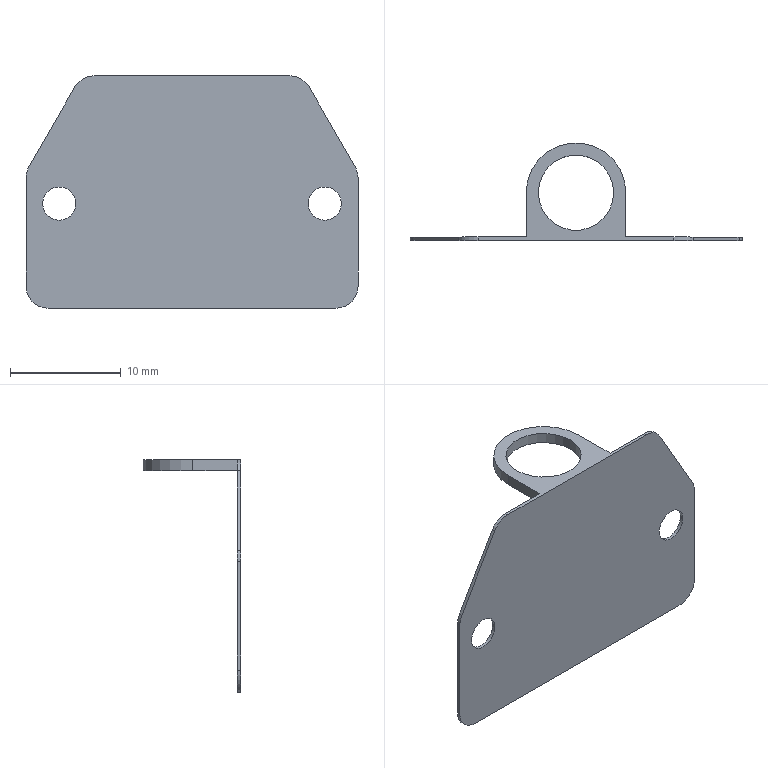Part | STEP file | 1 solid | 21 faces | box 30 x 8.8 x 21 mm | volume 202.601 mm3 | plane 11 | cylinder 10 | commonest cylinder face diameters 4 x6 3 x2 6.8 x1 9 x1